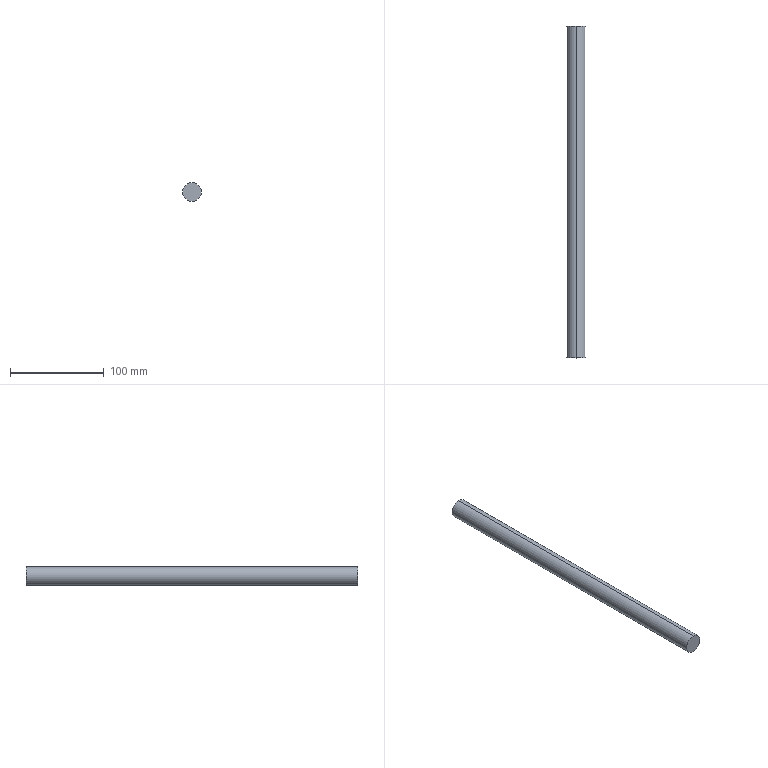Part | 1 solid | 4 faces | box 20 x 355 x 20 mm | volume 111527 mm3 | cylinder 2 | plane 2 | commonest cylinder face diameters 20 x2
STEP:
#1=CARTESIAN_POINT('',(0.,0.,0.));
#2=DIRECTION('',(0.,0.,1.));
#3=DIRECTION('',(1.,0.,0.));
#4=AXIS2_PLACEMENT_3D('',#1,#2,#3);
#5=CARTESIAN_POINT('',(-359.028,254.5,-290.55));
#6=VERTEX_POINT('',#5);
#7=CARTESIAN_POINT('',(-359.028,-100.5,-290.55));
#8=VERTEX_POINT('',#7);
#9=CARTESIAN_POINT('',(-359.028,254.5,-290.55));
#10=DIRECTION('',(0.,-1.,0.));
#11=VECTOR('',#10,1.);
#12=LINE('',#9,#11);
#13=CARTESIAN_POINT('',(-359.028,254.5,-300.55));
#14=DIRECTION('',(0.,-1.,0.));
#15=DIRECTION('',(1.,0.,0.));
#16=AXIS2_PLACEMENT_3D('',#13,#14,#15);
#17=CYLINDRICAL_SURFACE('',#16,10.);
#18=CARTESIAN_POINT('',(1.571,0.));
#19=DIRECTION('',(0.,1.));
#20=VECTOR('',#19,1.);
#21=LINE('',#18,#20);
#22=(GEOMETRIC_REPRESENTATION_CONTEXT(2)PARAMETRIC_REPRESENTATION_CONTEXT()REPRESENTATION_CONTEXT('',''));
#23=DEFINITIONAL_REPRESENTATION('',(#21),#22);
#24=PCURVE('',#17,#23);
#25=CARTESIAN_POINT('',(-359.028,254.5,-300.55));
#26=DIRECTION('',(0.,-1.,0.));
#27=DIRECTION('',(-1.,0.,0.));
#28=AXIS2_PLACEMENT_3D('',#25,#26,#27);
#29=CYLINDRICAL_SURFACE('',#28,10.);
#30=CARTESIAN_POINT('',(4.712,0.));
#31=DIRECTION('',(0.,1.));
#32=VECTOR('',#31,1.);
#33=LINE('',#30,#32);
#34=(GEOMETRIC_REPRESENTATION_CONTEXT(2)PARAMETRIC_REPRESENTATION_CONTEXT()REPRESENTATION_CONTEXT('',''));
#35=DEFINITIONAL_REPRESENTATION('',(#33),#34);
#36=PCURVE('',#29,#35);
#37=SURFACE_CURVE('',#12,(#24,#36),.PCURVE_S1.);
#38=EDGE_CURVE('',#6,#8,#37,.T.);
#39=ORIENTED_EDGE('',*,*,#38,.F.);
#40=CARTESIAN_POINT('',(-359.028,254.5,-310.55));
#41=VERTEX_POINT('',#40);
#42=CARTESIAN_POINT('',(-359.028,254.5,-300.55));
#43=DIRECTION('',(0.,1.,0.));
#44=DIRECTION('',(0.,0.,-1.));
#45=AXIS2_PLACEMENT_3D('',#42,#43,#44);
#46=CIRCLE('',#45,10.);
#47=CARTESIAN_POINT('',(4.712,0.));
#48=DIRECTION('',(-1.,0.));
#49=VECTOR('',#48,1.);
#50=LINE('',#47,#49);
#51=(GEOMETRIC_REPRESENTATION_CONTEXT(2)PARAMETRIC_REPRESENTATION_CONTEXT()REPRESENTATION_CONTEXT('',''));
#52=DEFINITIONAL_REPRESENTATION('',(#50),#51);
#53=PCURVE('',#17,#52);
#54=CARTESIAN_POINT('',(-359.028,254.5,-300.55));
#55=DIRECTION('',(0.,1.,0.));
#56=DIRECTION('',(0.,0.,1.));
#57=AXIS2_PLACEMENT_3D('',#54,#55,#56);
#58=PLANE('',#57);
#59=CARTESIAN_POINT('',(0.,0.));
#60=DIRECTION('',(-1.,0.));
#61=AXIS2_PLACEMENT_2D('',#59,#60);
#62=CIRCLE('',#61,10.);
#63=(GEOMETRIC_REPRESENTATION_CONTEXT(2)PARAMETRIC_REPRESENTATION_CONTEXT()REPRESENTATION_CONTEXT('',''));
#64=DEFINITIONAL_REPRESENTATION('',(#62),#63);
#65=PCURVE('',#58,#64);
#66=SURFACE_CURVE('',#46,(#53,#65),.PCURVE_S1.);
#67=EDGE_CURVE('',#41,#6,#66,.T.);
#68=ORIENTED_EDGE('',*,*,#67,.F.);
#69=CARTESIAN_POINT('',(-359.028,-100.5,-310.55));
#70=VERTEX_POINT('',#69);
#71=CARTESIAN_POINT('',(-359.028,254.5,-310.55));
#72=DIRECTION('',(0.,-1.,0.));
#73=VECTOR('',#72,1.);
#74=LINE('',#71,#73);
#75=CARTESIAN_POINT('',(4.712,0.));
#76=DIRECTION('',(0.,1.));
#77=VECTOR('',#76,1.);
#78=LINE('',#75,#77);
#79=(GEOMETRIC_REPRESENTATION_CONTEXT(2)PARAMETRIC_REPRESENTATION_CONTEXT()REPRESENTATION_CONTEXT('',''));
#80=DEFINITIONAL_REPRESENTATION('',(#78),#79);
#81=PCURVE('',#17,#80);
#82=CARTESIAN_POINT('',(1.571,0.));
#83=DIRECTION('',(0.,1.));
#84=VECTOR('',#83,1.);
#85=LINE('',#82,#84);
#86=(GEOMETRIC_REPRESENTATION_CONTEXT(2)PARAMETRIC_REPRESENTATION_CONTEXT()REPRESENTATION_CONTEXT('',''));
#87=DEFINITIONAL_REPRESENTATION('',(#85),#86);
#88=PCURVE('',#29,#87);
#89=SURFACE_CURVE('',#74,(#81,#88),.PCURVE_S1.);
#90=EDGE_CURVE('',#41,#70,#89,.T.);
#91=ORIENTED_EDGE('',*,*,#90,.T.);
#92=CARTESIAN_POINT('',(-359.028,-100.5,-300.55));
#93=DIRECTION('',(0.,1.,0.));
#94=DIRECTION('',(0.,0.,-1.));
#95=AXIS2_PLACEMENT_3D('',#92,#93,#94);
#96=CIRCLE('',#95,10.);
#97=CARTESIAN_POINT('',(4.712,355.));
#98=DIRECTION('',(-1.,0.));
#99=VECTOR('',#98,1.);
#100=LINE('',#97,#99);
#101=(GEOMETRIC_REPRESENTATION_CONTEXT(2)PARAMETRIC_REPRESENTATION_CONTEXT()REPRESENTATION_CONTEXT('',''));
#102=DEFINITIONAL_REPRESENTATION('',(#100),#101);
#103=PCURVE('',#17,#102);
#104=CARTESIAN_POINT('',(-239.028,-100.5,-300.55));
#105=DIRECTION('',(0.,1.,0.));
#106=DIRECTION('',(0.,0.,1.));
#107=AXIS2_PLACEMENT_3D('',#104,#105,#106);
#108=PLANE('',#107);
#109=CARTESIAN_POINT('',(0.,-120.));
#110=DIRECTION('',(-1.,0.));
#111=AXIS2_PLACEMENT_2D('',#109,#110);
#112=CIRCLE('',#111,10.);
#113=(GEOMETRIC_REPRESENTATION_CONTEXT(2)PARAMETRIC_REPRESENTATION_CONTEXT()REPRESENTATION_CONTEXT('',''));
#114=DEFINITIONAL_REPRESENTATION('',(#112),#113);
#115=PCURVE('',#108,#114);
#116=SURFACE_CURVE('',#96,(#103,#115),.PCURVE_S1.);
#117=EDGE_CURVE('',#70,#8,#116,.T.);
#118=ORIENTED_EDGE('',*,*,#117,.T.);
#119=EDGE_LOOP('',(#39,#68,#91,#118));
#120=FACE_BOUND('',#119,.T.);
#121=ADVANCED_FACE('',(#120),#17,.T.);
#122=ORIENTED_EDGE('',*,*,#67,.T.);
#123=CARTESIAN_POINT('',(-359.028,254.5,-300.55));
#124=DIRECTION('',(0.,1.,0.));
#125=DIRECTION('',(0.,0.,-1.));
#126=AXIS2_PLACEMENT_3D('',#123,#124,#125);
#127=CIRCLE('',#126,10.);
#128=CARTESIAN_POINT('',(0.,0.));
#129=DIRECTION('',(-1.,0.));
#130=AXIS2_PLACEMENT_2D('',#128,#129);
#131=CIRCLE('',#130,10.);
#132=(GEOMETRIC_REPRESENTATION_CONTEXT(2)PARAMETRIC_REPRESENTATION_CONTEXT()REPRESENTATION_CONTEXT('',''));
#133=DEFINITIONAL_REPRESENTATION('',(#131),#132);
#134=PCURVE('',#58,#133);
#135=CARTESIAN_POINT('',(7.854,0.));
#136=DIRECTION('',(-1.,0.));
#137=VECTOR('',#136,1.);
#138=LINE('',#135,#137);
#139=(GEOMETRIC_REPRESENTATION_CONTEXT(2)PARAMETRIC_REPRESENTATION_CONTEXT()REPRESENTATION_CONTEXT('',''));
#140=DEFINITIONAL_REPRESENTATION('',(#138),#139);
#141=PCURVE('',#29,#140);
#142=SURFACE_CURVE('',#127,(#134,#141),.PCURVE_S1.);
#143=EDGE_CURVE('',#6,#41,#142,.T.);
#144=ORIENTED_EDGE('',*,*,#143,.T.);
#145=EDGE_LOOP('',(#122,#144));
#146=FACE_BOUND('',#145,.T.);
#147=ADVANCED_FACE('',(#146),#58,.T.);
#148=CARTESIAN_POINT('',(-359.028,-100.5,-300.55));
#149=DIRECTION('',(0.,1.,0.));
#150=DIRECTION('',(0.,0.,-1.));
#151=AXIS2_PLACEMENT_3D('',#148,#149,#150);
#152=CIRCLE('',#151,10.);
#153=CARTESIAN_POINT('',(0.,-120.));
#154=DIRECTION('',(-1.,0.));
#155=AXIS2_PLACEMENT_2D('',#153,#154);
#156=CIRCLE('',#155,10.);
#157=(GEOMETRIC_REPRESENTATION_CONTEXT(2)PARAMETRIC_REPRESENTATION_CONTEXT()REPRESENTATION_CONTEXT('',''));
#158=DEFINITIONAL_REPRESENTATION('',(#156),#157);
#159=PCURVE('',#108,#158);
#160=CARTESIAN_POINT('',(7.854,355.));
#161=DIRECTION('',(-1.,0.));
#162=VECTOR('',#161,1.);
#163=LINE('',#160,#162);
#164=(GEOMETRIC_REPRESENTATION_CONTEXT(2)PARAMETRIC_REPRESENTATION_CONTEXT()REPRESENTATION_CONTEXT('',''));
#165=DEFINITIONAL_REPRESENTATION('',(#163),#164);
#166=PCURVE('',#29,#165);
#167=SURFACE_CURVE('',#152,(#159,#166),.PCURVE_S1.);
#168=EDGE_CURVE('',#8,#70,#167,.T.);
#169=ORIENTED_EDGE('',*,*,#168,.F.);
#170=ORIENTED_EDGE('',*,*,#117,.F.);
#171=EDGE_LOOP('',(#169,#170));
#172=FACE_BOUND('',#171,.T.);
#173=ADVANCED_FACE('',(#172),#108,.F.);
#174=ORIENTED_EDGE('',*,*,#38,.T.);
#175=ORIENTED_EDGE('',*,*,#168,.T.);
#176=ORIENTED_EDGE('',*,*,#90,.F.);
#177=ORIENTED_EDGE('',*,*,#143,.F.);
#178=EDGE_LOOP('',(#174,#175,#176,#177));
#179=FACE_BOUND('',#178,.T.);
#180=ADVANCED_FACE('',(#179),#29,.T.);
#181=CLOSED_SHELL('',(#121,#147,#173,#180));
#182=MANIFOLD_SOLID_BREP('',#181);
#183=(LENGTH_UNIT()NAMED_UNIT(*)SI_UNIT(.MILLI.,.METRE.));
#184=UNCERTAINTY_MEASURE_WITH_UNIT(LENGTH_MEASURE(0.0000001),#183,'','');
#185=(NAMED_UNIT(*)PLANE_ANGLE_UNIT()SI_UNIT($,.RADIAN.));
#186=(NAMED_UNIT(*)SI_UNIT($,.STERADIAN.)SOLID_ANGLE_UNIT());
#187=(GEOMETRIC_REPRESENTATION_CONTEXT(3)GLOBAL_UNCERTAINTY_ASSIGNED_CONTEXT((#184))GLOBAL_UNIT_ASSIGNED_CONTEXT((#183,#185,#186))REPRESENTATION_CONTEXT('',''));
#188=ADVANCED_BREP_SHAPE_REPRESENTATION('',(#4,#182),#187);